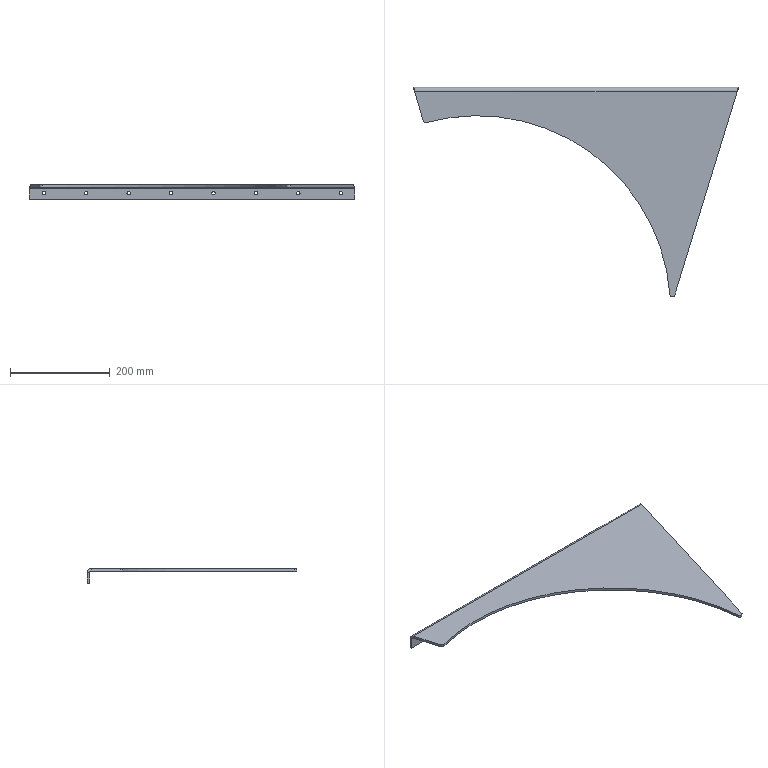Part | SolidWorks | features EdgeFlange 1, Fillet 1, FlatPattern 1, HoleWzd 1, LPattern 1, SMBaseFlange 1, SheetMetal 1 | 1 solid | 48 faces | box 651.256 x 419.882 x 30 mm | volume 531655 mm3 | cylinder 21 | cone 16 | plane 9 | spline 2 | commonest cylinder face diameters 7 x16 10 x2 6 x1 16 x1 775 x1